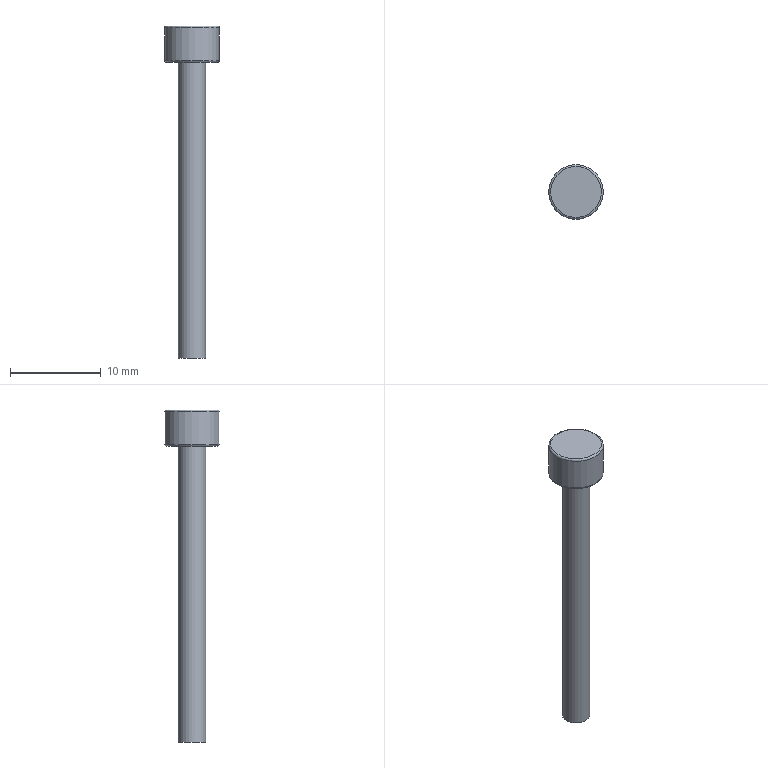Part | STEP file | 200 mesh_id94_xmt | 1 solid | 7 faces | box 6 x 6 x 36.5 mm | volume 342.508 mm3 | plane 3 | cylinder 2 | torus 2 | commonest cylinder face diameters 3 x1 6 x1
STEP:
#1=CARTESIAN_POINT('',(-17010.021,-3997.769,116.258));
#2=VERTEX_POINT('',#1);
#3=CARTESIAN_POINT('',(-17012.821,-3997.769,116.258));
#4=DIRECTION('',(0.,0.,1.));
#5=DIRECTION('',(1.,0.,0.));
#6=AXIS2_PLACEMENT_3D('',#3,#4,#5);
#7=CIRCLE('',#6,2.8);
#8=EDGE_CURVE('',#2,#2,#7,.T.);
#9=ORIENTED_EDGE('',*,*,#8,.T.);
#10=EDGE_LOOP('',(#9));
#11=FACE_OUTER_BOUND('',#10,.T.);
#12=CARTESIAN_POINT('',(-17012.821,-3997.769,116.258));
#13=DIRECTION('',(0.,0.,1.));
#14=DIRECTION('',(1.,0.,0.));
#15=AXIS2_PLACEMENT_3D('',#12,#13,#14);
#16=PLANE('',#15);
#17=ADVANCED_FACE('',(#11),#16,.T.);
#18=CARTESIAN_POINT('',(-17015.621,-3997.769,112.258));
#19=VERTEX_POINT('',#18);
#20=CARTESIAN_POINT('',(-17012.821,-3997.769,112.258));
#21=DIRECTION('',(0.,0.,-1.));
#22=DIRECTION('',(-1.,0.,0.));
#23=AXIS2_PLACEMENT_3D('',#20,#21,#22);
#24=CIRCLE('',#23,2.8);
#25=EDGE_CURVE('',#19,#19,#24,.T.);
#26=ORIENTED_EDGE('',*,*,#25,.T.);
#27=EDGE_LOOP('',(#26));
#28=FACE_BOUND('',#27,.T.);
#29=CARTESIAN_POINT('',(-17011.321,-3997.769,112.258));
#30=VERTEX_POINT('',#29);
#31=CARTESIAN_POINT('',(-17012.821,-3997.769,112.258));
#32=DIRECTION('',(0.,0.,1.));
#33=DIRECTION('',(1.,0.,0.));
#34=AXIS2_PLACEMENT_3D('',#31,#32,#33);
#35=CIRCLE('',#34,1.5);
#36=EDGE_CURVE('',#30,#30,#35,.T.);
#37=ORIENTED_EDGE('',*,*,#36,.T.);
#38=EDGE_LOOP('',(#37));
#39=FACE_BOUND('',#38,.T.);
#40=CARTESIAN_POINT('',(-17012.821,-3997.769,112.258));
#41=DIRECTION('',(0.,0.,-1.));
#42=DIRECTION('',(-1.,0.,0.));
#43=AXIS2_PLACEMENT_3D('',#40,#41,#42);
#44=PLANE('',#43);
#45=ADVANCED_FACE('',(#28,#39),#44,.T.);
#46=CARTESIAN_POINT('',(-17015.821,-3997.769,112.458));
#47=VERTEX_POINT('',#46);
#48=CARTESIAN_POINT('',(-17012.821,-3997.769,112.458));
#49=DIRECTION('',(0.,0.,1.));
#50=DIRECTION('',(-1.,0.,0.));
#51=AXIS2_PLACEMENT_3D('',#48,#49,#50);
#52=CIRCLE('',#51,3.);
#53=EDGE_CURVE('',#47,#47,#52,.T.);
#54=ORIENTED_EDGE('',*,*,#53,.T.);
#55=EDGE_LOOP('',(#54));
#56=FACE_BOUND('',#55,.T.);
#57=CARTESIAN_POINT('',(-17009.821,-3997.769,116.058));
#58=VERTEX_POINT('',#57);
#59=CARTESIAN_POINT('',(-17012.821,-3997.769,116.058));
#60=DIRECTION('',(0.,0.,-1.));
#61=DIRECTION('',(1.,0.,0.));
#62=AXIS2_PLACEMENT_3D('',#59,#60,#61);
#63=CIRCLE('',#62,3.);
#64=EDGE_CURVE('',#58,#58,#63,.T.);
#65=ORIENTED_EDGE('',*,*,#64,.T.);
#66=EDGE_LOOP('',(#65));
#67=FACE_BOUND('',#66,.T.);
#68=CARTESIAN_POINT('',(-17012.821,-3997.769,112.258));
#69=DIRECTION('',(0.,0.,1.));
#70=DIRECTION('',(1.,0.,0.));
#71=AXIS2_PLACEMENT_3D('',#68,#69,#70);
#72=CYLINDRICAL_SURFACE('',#71,3.);
#73=ADVANCED_FACE('',(#56,#67),#72,.T.);
#74=CARTESIAN_POINT('',(-17011.321,-3997.769,79.758));
#75=VERTEX_POINT('',#74);
#76=CARTESIAN_POINT('',(-17012.821,-3997.769,79.758));
#77=DIRECTION('',(0.,0.,1.));
#78=DIRECTION('',(1.,0.,0.));
#79=AXIS2_PLACEMENT_3D('',#76,#77,#78);
#80=CIRCLE('',#79,1.5);
#81=EDGE_CURVE('',#75,#75,#80,.T.);
#82=ORIENTED_EDGE('',*,*,#81,.T.);
#83=EDGE_LOOP('',(#82));
#84=FACE_BOUND('',#83,.T.);
#85=ORIENTED_EDGE('',*,*,#36,.F.);
#86=EDGE_LOOP('',(#85));
#87=FACE_BOUND('',#86,.T.);
#88=CARTESIAN_POINT('',(-17012.821,-3997.769,75.258));
#89=DIRECTION('',(0.,0.,1.));
#90=DIRECTION('',(1.,0.,0.));
#91=AXIS2_PLACEMENT_3D('',#88,#89,#90);
#92=CYLINDRICAL_SURFACE('',#91,1.5);
#93=ADVANCED_FACE('',(#84,#87),#92,.T.);
#94=ORIENTED_EDGE('',*,*,#81,.F.);
#95=EDGE_LOOP('',(#94));
#96=FACE_OUTER_BOUND('',#95,.T.);
#97=CARTESIAN_POINT('',(-17012.821,-3997.769,79.758));
#98=DIRECTION('',(0.,0.,1.));
#99=DIRECTION('',(1.,0.,0.));
#100=AXIS2_PLACEMENT_3D('',#97,#98,#99);
#101=PLANE('',#100);
#102=ADVANCED_FACE('',(#96),#101,.F.);
#103=ORIENTED_EDGE('',*,*,#25,.F.);
#104=EDGE_LOOP('',(#103));
#105=FACE_BOUND('',#104,.T.);
#106=ORIENTED_EDGE('',*,*,#53,.F.);
#107=EDGE_LOOP('',(#106));
#108=FACE_BOUND('',#107,.T.);
#109=CARTESIAN_POINT('',(-17012.821,-3997.769,112.458));
#110=DIRECTION('',(0.,0.,-1.));
#111=DIRECTION('',(-1.,0.,0.));
#112=AXIS2_PLACEMENT_3D('',#109,#110,#111);
#113=TOROIDAL_SURFACE('',#112,2.8,0.2);
#114=ADVANCED_FACE('',(#105,#108),#113,.T.);
#115=ORIENTED_EDGE('',*,*,#8,.F.);
#116=EDGE_LOOP('',(#115));
#117=FACE_BOUND('',#116,.T.);
#118=ORIENTED_EDGE('',*,*,#64,.F.);
#119=EDGE_LOOP('',(#118));
#120=FACE_BOUND('',#119,.T.);
#121=CARTESIAN_POINT('',(-17012.821,-3997.769,116.058));
#122=DIRECTION('',(0.,0.,1.));
#123=DIRECTION('',(1.,0.,0.));
#124=AXIS2_PLACEMENT_3D('',#121,#122,#123);
#125=TOROIDAL_SURFACE('',#124,2.8,0.2);
#126=ADVANCED_FACE('',(#117,#120),#125,.T.);
#127=CLOSED_SHELL('',(#17,#45,#73,#93,#102,#114,#126));
#128=MANIFOLD_SOLID_BREP('',#127);
#129=(LENGTH_UNIT()NAMED_UNIT(*)SI_UNIT(.MILLI.,.METRE.));
#130=UNCERTAINTY_MEASURE_WITH_UNIT(LENGTH_MEASURE(0.00002),#129,'','');
#131=(NAMED_UNIT(*)PLANE_ANGLE_UNIT()SI_UNIT($,.RADIAN.));
#132=PLANE_ANGLE_MEASURE_WITH_UNIT(PLANE_ANGLE_MEASURE(0.01745),#131);
#133=DIMENSIONAL_EXPONENTS(0.,0.,0.,0.,0.,0.,0.);
#134=(CONVERSION_BASED_UNIT('DEGREE',#132)NAMED_UNIT(#133)PLANE_ANGLE_UNIT());
#135=(NAMED_UNIT(*)SI_UNIT($,.STERADIAN.)SOLID_ANGLE_UNIT());
#136=(GEOMETRIC_REPRESENTATION_CONTEXT(3)GLOBAL_UNCERTAINTY_ASSIGNED_CONTEXT((#130))GLOBAL_UNIT_ASSIGNED_CONTEXT((#129,#134,#135))REPRESENTATION_CONTEXT('',''));
#137=ADVANCED_BREP_SHAPE_REPRESENTATION('',(#128),#136);